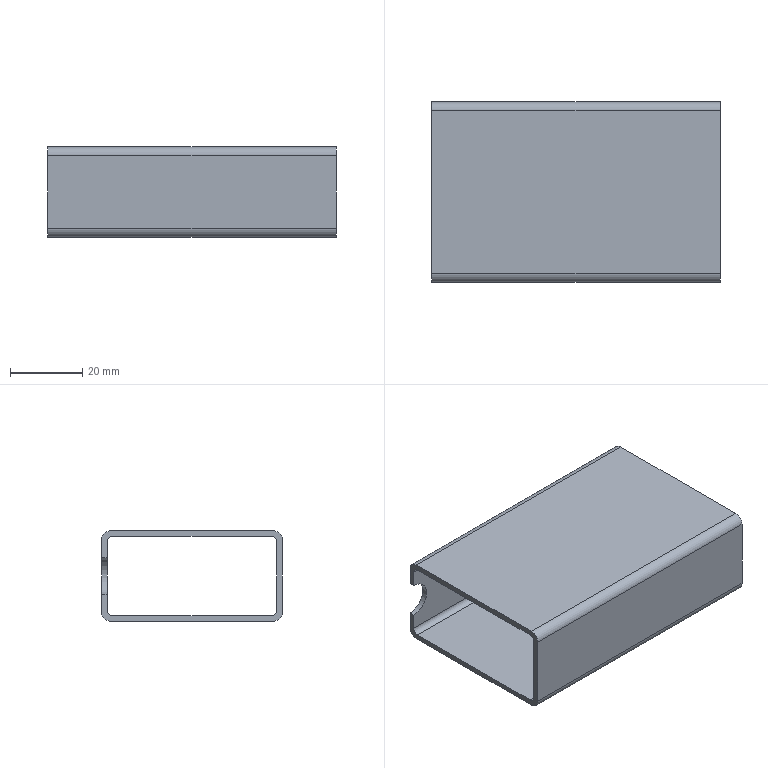Part | STEP file | 6150507 | 1 solid | 19 faces | box 80 x 50 x 25 mm | volume 16946 mm3 | plane 10 | cylinder 9 | commonest cylinder face diameters 3 x4 5 x4 10 x1
STEP:
#1=CARTESIAN_POINT('',(-40.,23.5,-9.5));
#2=VERTEX_POINT('',#1);
#3=CARTESIAN_POINT('',(-40.,23.5,-5.));
#4=VERTEX_POINT('',#3);
#5=CARTESIAN_POINT('',(-40.,23.5,9.5));
#6=DIRECTION('',(0.,0.,1.));
#7=VECTOR('',#6,1000.);
#8=LINE('',#5,#7);
#9=EDGE_CURVE('',#2,#4,#8,.T.);
#10=ORIENTED_EDGE('',*,*,#9,.T.);
#11=CARTESIAN_POINT('',(-40.,25.,-5.));
#12=VERTEX_POINT('',#11);
#13=CARTESIAN_POINT('',(-40.,15.,-5.));
#14=DIRECTION('',(0.,1.,0.));
#15=VECTOR('',#14,1000.);
#16=LINE('',#13,#15);
#17=EDGE_CURVE('',#4,#12,#16,.T.);
#18=ORIENTED_EDGE('',*,*,#17,.T.);
#19=CARTESIAN_POINT('',(-40.,25.,-10.));
#20=VERTEX_POINT('',#19);
#21=CARTESIAN_POINT('',(-40.,25.,12.5));
#22=DIRECTION('',(0.,0.,-1.));
#23=VECTOR('',#22,1000.);
#24=LINE('',#21,#23);
#25=EDGE_CURVE('',#12,#20,#24,.T.);
#26=ORIENTED_EDGE('',*,*,#25,.T.);
#27=CARTESIAN_POINT('',(-40.,22.5,-12.5));
#28=VERTEX_POINT('',#27);
#29=CARTESIAN_POINT('',(-40.,22.5,-10.));
#30=DIRECTION('',(-1.,0.,0.));
#31=DIRECTION('',(0.,1.,0.));
#32=AXIS2_PLACEMENT_3D('',#29,#30,#31);
#33=CIRCLE('',#32,2.5);
#34=EDGE_CURVE('',#20,#28,#33,.T.);
#35=ORIENTED_EDGE('',*,*,#34,.T.);
#36=CARTESIAN_POINT('',(-40.,-22.5,-12.5));
#37=VERTEX_POINT('',#36);
#38=CARTESIAN_POINT('',(-40.,25.,-12.5));
#39=DIRECTION('',(0.,-1.,0.));
#40=VECTOR('',#39,1000.);
#41=LINE('',#38,#40);
#42=EDGE_CURVE('',#28,#37,#41,.T.);
#43=ORIENTED_EDGE('',*,*,#42,.T.);
#44=CARTESIAN_POINT('',(-40.,-25.,-10.));
#45=VERTEX_POINT('',#44);
#46=CARTESIAN_POINT('',(-40.,-22.5,-10.));
#47=DIRECTION('',(-1.,0.,0.));
#48=DIRECTION('',(0.,1.,0.));
#49=AXIS2_PLACEMENT_3D('',#46,#47,#48);
#50=CIRCLE('',#49,2.5);
#51=EDGE_CURVE('',#37,#45,#50,.T.);
#52=ORIENTED_EDGE('',*,*,#51,.T.);
#53=CARTESIAN_POINT('',(-40.,-25.,10.));
#54=VERTEX_POINT('',#53);
#55=CARTESIAN_POINT('',(-40.,-25.,12.5));
#56=DIRECTION('',(0.,0.,-1.));
#57=VECTOR('',#56,1000.);
#58=LINE('',#55,#57);
#59=EDGE_CURVE('',#54,#45,#58,.T.);
#60=ORIENTED_EDGE('',*,*,#59,.F.);
#61=CARTESIAN_POINT('',(-40.,-22.5,12.5));
#62=VERTEX_POINT('',#61);
#63=CARTESIAN_POINT('',(-40.,-22.5,10.));
#64=DIRECTION('',(-1.,0.,0.));
#65=DIRECTION('',(0.,1.,0.));
#66=AXIS2_PLACEMENT_3D('',#63,#64,#65);
#67=CIRCLE('',#66,2.5);
#68=EDGE_CURVE('',#54,#62,#67,.T.);
#69=ORIENTED_EDGE('',*,*,#68,.T.);
#70=CARTESIAN_POINT('',(-40.,22.5,12.5));
#71=VERTEX_POINT('',#70);
#72=CARTESIAN_POINT('',(-40.,25.,12.5));
#73=DIRECTION('',(0.,-1.,0.));
#74=VECTOR('',#73,1000.);
#75=LINE('',#72,#74);
#76=EDGE_CURVE('',#71,#62,#75,.T.);
#77=ORIENTED_EDGE('',*,*,#76,.F.);
#78=CARTESIAN_POINT('',(-40.,25.,10.));
#79=VERTEX_POINT('',#78);
#80=CARTESIAN_POINT('',(-40.,22.5,10.));
#81=DIRECTION('',(-1.,0.,0.));
#82=DIRECTION('',(0.,1.,0.));
#83=AXIS2_PLACEMENT_3D('',#80,#81,#82);
#84=CIRCLE('',#83,2.5);
#85=EDGE_CURVE('',#71,#79,#84,.T.);
#86=ORIENTED_EDGE('',*,*,#85,.T.);
#87=CARTESIAN_POINT('',(-40.,25.,5.));
#88=VERTEX_POINT('',#87);
#89=CARTESIAN_POINT('',(-40.,25.,12.5));
#90=DIRECTION('',(0.,0.,-1.));
#91=VECTOR('',#90,1000.);
#92=LINE('',#89,#91);
#93=EDGE_CURVE('',#79,#88,#92,.T.);
#94=ORIENTED_EDGE('',*,*,#93,.T.);
#95=CARTESIAN_POINT('',(-40.,23.5,5.));
#96=VERTEX_POINT('',#95);
#97=CARTESIAN_POINT('',(-40.,15.,5.));
#98=DIRECTION('',(0.,-1.,0.));
#99=VECTOR('',#98,1000.);
#100=LINE('',#97,#99);
#101=EDGE_CURVE('',#88,#96,#100,.T.);
#102=ORIENTED_EDGE('',*,*,#101,.T.);
#103=CARTESIAN_POINT('',(-40.,23.5,9.5));
#104=VERTEX_POINT('',#103);
#105=CARTESIAN_POINT('',(-40.,23.5,9.5));
#106=DIRECTION('',(0.,0.,1.));
#107=VECTOR('',#106,1000.);
#108=LINE('',#105,#107);
#109=EDGE_CURVE('',#96,#104,#108,.T.);
#110=ORIENTED_EDGE('',*,*,#109,.T.);
#111=CARTESIAN_POINT('',(-40.,22.,11.));
#112=VERTEX_POINT('',#111);
#113=CARTESIAN_POINT('',(-40.,22.,9.5));
#114=DIRECTION('',(1.,0.,0.));
#115=DIRECTION('',(0.,1.,0.));
#116=AXIS2_PLACEMENT_3D('',#113,#114,#115);
#117=CIRCLE('',#116,1.5);
#118=EDGE_CURVE('',#104,#112,#117,.T.);
#119=ORIENTED_EDGE('',*,*,#118,.T.);
#120=CARTESIAN_POINT('',(-40.,-22.,11.));
#121=VERTEX_POINT('',#120);
#122=CARTESIAN_POINT('',(-40.,22.,11.));
#123=DIRECTION('',(0.,-1.,0.));
#124=VECTOR('',#123,1000.);
#125=LINE('',#122,#124);
#126=EDGE_CURVE('',#112,#121,#125,.T.);
#127=ORIENTED_EDGE('',*,*,#126,.T.);
#128=CARTESIAN_POINT('',(-40.,-23.5,9.5));
#129=VERTEX_POINT('',#128);
#130=CARTESIAN_POINT('',(-40.,-22.,9.5));
#131=DIRECTION('',(1.,0.,0.));
#132=DIRECTION('',(0.,1.,0.));
#133=AXIS2_PLACEMENT_3D('',#130,#131,#132);
#134=CIRCLE('',#133,1.5);
#135=EDGE_CURVE('',#121,#129,#134,.T.);
#136=ORIENTED_EDGE('',*,*,#135,.T.);
#137=CARTESIAN_POINT('',(-40.,-23.5,-9.5));
#138=VERTEX_POINT('',#137);
#139=CARTESIAN_POINT('',(-40.,-23.5,9.5));
#140=DIRECTION('',(0.,0.,-1.));
#141=VECTOR('',#140,1000.);
#142=LINE('',#139,#141);
#143=EDGE_CURVE('',#129,#138,#142,.T.);
#144=ORIENTED_EDGE('',*,*,#143,.T.);
#145=CARTESIAN_POINT('',(-40.,-22.,-11.));
#146=VERTEX_POINT('',#145);
#147=CARTESIAN_POINT('',(-40.,-22.,-9.5));
#148=DIRECTION('',(1.,0.,0.));
#149=DIRECTION('',(0.,1.,0.));
#150=AXIS2_PLACEMENT_3D('',#147,#148,#149);
#151=CIRCLE('',#150,1.5);
#152=EDGE_CURVE('',#138,#146,#151,.T.);
#153=ORIENTED_EDGE('',*,*,#152,.T.);
#154=CARTESIAN_POINT('',(-40.,22.,-11.));
#155=VERTEX_POINT('',#154);
#156=CARTESIAN_POINT('',(-40.,22.,-11.));
#157=DIRECTION('',(0.,1.,0.));
#158=VECTOR('',#157,1000.);
#159=LINE('',#156,#158);
#160=EDGE_CURVE('',#146,#155,#159,.T.);
#161=ORIENTED_EDGE('',*,*,#160,.T.);
#162=CARTESIAN_POINT('',(-40.,22.,-9.5));
#163=DIRECTION('',(1.,0.,0.));
#164=DIRECTION('',(0.,-1.,0.));
#165=AXIS2_PLACEMENT_3D('',#162,#163,#164);
#166=CIRCLE('',#165,1.5);
#167=EDGE_CURVE('',#155,#2,#166,.T.);
#168=ORIENTED_EDGE('',*,*,#167,.T.);
#169=EDGE_LOOP('',(#10,#18,#26,#35,#43,#52,#60,#69,#77,#86,#94,#102,#110,#119,#127,#136,#144,#153,#161,#168));
#170=FACE_OUTER_BOUND('',#169,.T.);
#171=CARTESIAN_POINT('',(-40.,25.,12.5));
#172=DIRECTION('',(1.,0.,0.));
#173=DIRECTION('',(0.,1.,0.));
#174=AXIS2_PLACEMENT_3D('',#171,#172,#173);
#175=PLANE('',#174);
#176=ADVANCED_FACE('',(#170),#175,.F.);
#177=CARTESIAN_POINT('',(40.,-25.,10.));
#178=VERTEX_POINT('',#177);
#179=CARTESIAN_POINT('',(40.,-25.,-10.));
#180=VERTEX_POINT('',#179);
#181=CARTESIAN_POINT('',(40.,-25.,12.5));
#182=DIRECTION('',(0.,0.,-1.));
#183=VECTOR('',#182,1000.);
#184=LINE('',#181,#183);
#185=EDGE_CURVE('',#178,#180,#184,.T.);
#186=ORIENTED_EDGE('',*,*,#185,.F.);
#187=CARTESIAN_POINT('',(-40.,-25.,10.));
#188=DIRECTION('',(-1.,0.,0.));
#189=VECTOR('',#188,1000.);
#190=LINE('',#187,#189);
#191=EDGE_CURVE('',#178,#54,#190,.T.);
#192=ORIENTED_EDGE('',*,*,#191,.T.);
#193=ORIENTED_EDGE('',*,*,#59,.T.);
#194=CARTESIAN_POINT('',(-40.,-25.,-10.));
#195=DIRECTION('',(1.,0.,0.));
#196=VECTOR('',#195,1000.);
#197=LINE('',#194,#196);
#198=EDGE_CURVE('',#45,#180,#197,.T.);
#199=ORIENTED_EDGE('',*,*,#198,.T.);
#200=EDGE_LOOP('',(#186,#192,#193,#199));
#201=FACE_OUTER_BOUND('',#200,.T.);
#202=CARTESIAN_POINT('',(-40.,-25.,12.5));
#203=DIRECTION('',(0.,1.,0.));
#204=DIRECTION('',(-1.,0.,0.));
#205=AXIS2_PLACEMENT_3D('',#202,#203,#204);
#206=PLANE('',#205);
#207=ADVANCED_FACE('',(#201),#206,.F.);
#208=CARTESIAN_POINT('',(40.,-23.5,9.5));
#209=VERTEX_POINT('',#208);
#210=CARTESIAN_POINT('',(40.,-23.5,-9.5));
#211=VERTEX_POINT('',#210);
#212=CARTESIAN_POINT('',(40.,-23.5,9.5));
#213=DIRECTION('',(0.,0.,-1.));
#214=VECTOR('',#213,1000.);
#215=LINE('',#212,#214);
#216=EDGE_CURVE('',#209,#211,#215,.T.);
#217=ORIENTED_EDGE('',*,*,#216,.F.);
#218=CARTESIAN_POINT('',(40.,-22.,11.));
#219=VERTEX_POINT('',#218);
#220=CARTESIAN_POINT('',(40.,-22.,9.5));
#221=DIRECTION('',(1.,0.,0.));
#222=DIRECTION('',(0.,1.,0.));
#223=AXIS2_PLACEMENT_3D('',#220,#221,#222);
#224=CIRCLE('',#223,1.5);
#225=EDGE_CURVE('',#219,#209,#224,.T.);
#226=ORIENTED_EDGE('',*,*,#225,.F.);
#227=CARTESIAN_POINT('',(40.,22.,11.));
#228=VERTEX_POINT('',#227);
#229=CARTESIAN_POINT('',(40.,22.,11.));
#230=DIRECTION('',(0.,-1.,0.));
#231=VECTOR('',#230,1000.);
#232=LINE('',#229,#231);
#233=EDGE_CURVE('',#228,#219,#232,.T.);
#234=ORIENTED_EDGE('',*,*,#233,.F.);
#235=CARTESIAN_POINT('',(40.,23.5,9.5));
#236=VERTEX_POINT('',#235);
#237=CARTESIAN_POINT('',(40.,22.,9.5));
#238=DIRECTION('',(1.,0.,0.));
#239=DIRECTION('',(0.,1.,0.));
#240=AXIS2_PLACEMENT_3D('',#237,#238,#239);
#241=CIRCLE('',#240,1.5);
#242=EDGE_CURVE('',#236,#228,#241,.T.);
#243=ORIENTED_EDGE('',*,*,#242,.F.);
#244=CARTESIAN_POINT('',(40.,23.5,-9.5));
#245=VERTEX_POINT('',#244);
#246=CARTESIAN_POINT('',(40.,23.5,9.5));
#247=DIRECTION('',(0.,0.,1.));
#248=VECTOR('',#247,1000.);
#249=LINE('',#246,#248);
#250=EDGE_CURVE('',#245,#236,#249,.T.);
#251=ORIENTED_EDGE('',*,*,#250,.F.);
#252=CARTESIAN_POINT('',(40.,22.,-11.));
#253=VERTEX_POINT('',#252);
#254=CARTESIAN_POINT('',(40.,22.,-9.5));
#255=DIRECTION('',(1.,0.,0.));
#256=DIRECTION('',(0.,-1.,0.));
#257=AXIS2_PLACEMENT_3D('',#254,#255,#256);
#258=CIRCLE('',#257,1.5);
#259=EDGE_CURVE('',#253,#245,#258,.T.);
#260=ORIENTED_EDGE('',*,*,#259,.F.);
#261=CARTESIAN_POINT('',(40.,-22.,-11.));
#262=VERTEX_POINT('',#261);
#263=CARTESIAN_POINT('',(40.,22.,-11.));
#264=DIRECTION('',(0.,1.,0.));
#265=VECTOR('',#264,1000.);
#266=LINE('',#263,#265);
#267=EDGE_CURVE('',#262,#253,#266,.T.);
#268=ORIENTED_EDGE('',*,*,#267,.F.);
#269=CARTESIAN_POINT('',(40.,-22.,-9.5));
#270=DIRECTION('',(1.,0.,0.));
#271=DIRECTION('',(0.,1.,0.));
#272=AXIS2_PLACEMENT_3D('',#269,#270,#271);
#273=CIRCLE('',#272,1.5);
#274=EDGE_CURVE('',#211,#262,#273,.T.);
#275=ORIENTED_EDGE('',*,*,#274,.F.);
#276=EDGE_LOOP('',(#217,#226,#234,#243,#251,#260,#268,#275));
#277=FACE_BOUND('',#276,.T.);
#278=CARTESIAN_POINT('',(40.,-22.5,12.5));
#279=VERTEX_POINT('',#278);
#280=CARTESIAN_POINT('',(40.,22.5,12.5));
#281=VERTEX_POINT('',#280);
#282=CARTESIAN_POINT('',(40.,25.,12.5));
#283=DIRECTION('',(0.,1.,0.));
#284=VECTOR('',#283,1000.);
#285=LINE('',#282,#284);
#286=EDGE_CURVE('',#279,#281,#285,.T.);
#287=ORIENTED_EDGE('',*,*,#286,.F.);
#288=CARTESIAN_POINT('',(40.,-22.5,10.));
#289=DIRECTION('',(1.,0.,0.));
#290=DIRECTION('',(0.,-1.,0.));
#291=AXIS2_PLACEMENT_3D('',#288,#289,#290);
#292=CIRCLE('',#291,2.5);
#293=EDGE_CURVE('',#279,#178,#292,.T.);
#294=ORIENTED_EDGE('',*,*,#293,.T.);
#295=ORIENTED_EDGE('',*,*,#185,.T.);
#296=CARTESIAN_POINT('',(40.,-22.5,-12.5));
#297=VERTEX_POINT('',#296);
#298=CARTESIAN_POINT('',(40.,-22.5,-10.));
#299=DIRECTION('',(1.,0.,0.));
#300=DIRECTION('',(0.,-1.,0.));
#301=AXIS2_PLACEMENT_3D('',#298,#299,#300);
#302=CIRCLE('',#301,2.5);
#303=EDGE_CURVE('',#180,#297,#302,.T.);
#304=ORIENTED_EDGE('',*,*,#303,.T.);
#305=CARTESIAN_POINT('',(40.,22.5,-12.5));
#306=VERTEX_POINT('',#305);
#307=CARTESIAN_POINT('',(40.,25.,-12.5));
#308=DIRECTION('',(0.,1.,0.));
#309=VECTOR('',#308,1000.);
#310=LINE('',#307,#309);
#311=EDGE_CURVE('',#297,#306,#310,.T.);
#312=ORIENTED_EDGE('',*,*,#311,.T.);
#313=CARTESIAN_POINT('',(40.,25.,-10.));
#314=VERTEX_POINT('',#313);
#315=CARTESIAN_POINT('',(40.,22.5,-10.));
#316=DIRECTION('',(1.,0.,0.));
#317=DIRECTION('',(0.,-1.,0.));
#318=AXIS2_PLACEMENT_3D('',#315,#316,#317);
#319=CIRCLE('',#318,2.5);
#320=EDGE_CURVE('',#306,#314,#319,.T.);
#321=ORIENTED_EDGE('',*,*,#320,.T.);
#322=CARTESIAN_POINT('',(40.,25.,10.));
#323=VERTEX_POINT('',#322);
#324=CARTESIAN_POINT('',(40.,25.,12.5));
#325=DIRECTION('',(0.,0.,-1.));
#326=VECTOR('',#325,1000.);
#327=LINE('',#324,#326);
#328=EDGE_CURVE('',#323,#314,#327,.T.);
#329=ORIENTED_EDGE('',*,*,#328,.F.);
#330=CARTESIAN_POINT('',(40.,22.5,10.));
#331=DIRECTION('',(1.,0.,0.));
#332=DIRECTION('',(0.,-1.,0.));
#333=AXIS2_PLACEMENT_3D('',#330,#331,#332);
#334=CIRCLE('',#333,2.5);
#335=EDGE_CURVE('',#323,#281,#334,.T.);
#336=ORIENTED_EDGE('',*,*,#335,.T.);
#337=EDGE_LOOP('',(#287,#294,#295,#304,#312,#321,#329,#336));
#338=FACE_OUTER_BOUND('',#337,.T.);
#339=CARTESIAN_POINT('',(40.,25.,12.5));
#340=DIRECTION('',(-1.,0.,0.));
#341=DIRECTION('',(0.,-1.,0.));
#342=AXIS2_PLACEMENT_3D('',#339,#340,#341);
#343=PLANE('',#342);
#344=ADVANCED_FACE('',(#277,#338),#343,.F.);
#345=ORIENTED_EDGE('',*,*,#25,.F.);
#346=CARTESIAN_POINT('',(-40.,25.,0.));
#347=DIRECTION('',(0.,1.,0.));
#348=DIRECTION('',(0.,0.,1.));
#349=AXIS2_PLACEMENT_3D('',#346,#347,#348);
#350=CIRCLE('',#349,5.);
#351=EDGE_CURVE('',#88,#12,#350,.T.);
#352=ORIENTED_EDGE('',*,*,#351,.F.);
#353=ORIENTED_EDGE('',*,*,#93,.F.);
#354=CARTESIAN_POINT('',(40.,25.,10.));
#355=DIRECTION('',(1.,0.,0.));
#356=VECTOR('',#355,1000.);
#357=LINE('',#354,#356);
#358=EDGE_CURVE('',#79,#323,#357,.T.);
#359=ORIENTED_EDGE('',*,*,#358,.T.);
#360=ORIENTED_EDGE('',*,*,#328,.T.);
#361=CARTESIAN_POINT('',(-40.,25.,-10.));
#362=DIRECTION('',(-1.,0.,0.));
#363=VECTOR('',#362,1000.);
#364=LINE('',#361,#363);
#365=EDGE_CURVE('',#314,#20,#364,.T.);
#366=ORIENTED_EDGE('',*,*,#365,.T.);
#367=EDGE_LOOP('',(#345,#352,#353,#359,#360,#366));
#368=FACE_OUTER_BOUND('',#367,.T.);
#369=CARTESIAN_POINT('',(-40.,25.,12.5));
#370=DIRECTION('',(0.,-1.,0.));
#371=DIRECTION('',(0.,0.,-1.));
#372=AXIS2_PLACEMENT_3D('',#369,#370,#371);
#373=PLANE('',#372);
#374=ADVANCED_FACE('',(#368),#373,.F.);
#375=ORIENTED_EDGE('',*,*,#76,.T.);
#376=CARTESIAN_POINT('',(40.,-22.5,12.5));
#377=DIRECTION('',(1.,0.,0.));
#378=VECTOR('',#377,1000.);
#379=LINE('',#376,#378);
#380=EDGE_CURVE('',#62,#279,#379,.T.);
#381=ORIENTED_EDGE('',*,*,#380,.T.);
#382=ORIENTED_EDGE('',*,*,#286,.T.);
#383=CARTESIAN_POINT('',(-40.,22.5,12.5));
#384=DIRECTION('',(-1.,0.,0.));
#385=VECTOR('',#384,1000.);
#386=LINE('',#383,#385);
#387=EDGE_CURVE('',#281,#71,#386,.T.);
#388=ORIENTED_EDGE('',*,*,#387,.T.);
#389=EDGE_LOOP('',(#375,#381,#382,#388));
#390=FACE_OUTER_BOUND('',#389,.T.);
#391=CARTESIAN_POINT('',(-40.,-25.,12.5));
#392=DIRECTION('',(0.,0.,1.));
#393=DIRECTION('',(1.,0.,0.));
#394=AXIS2_PLACEMENT_3D('',#391,#392,#393);
#395=PLANE('',#394);
#396=ADVANCED_FACE('',(#390),#395,.T.);
#397=ORIENTED_EDGE('',*,*,#311,.F.);
#398=CARTESIAN_POINT('',(-40.,-22.5,-12.5));
#399=DIRECTION('',(-1.,0.,0.));
#400=VECTOR('',#399,1000.);
#401=LINE('',#398,#400);
#402=EDGE_CURVE('',#297,#37,#401,.T.);
#403=ORIENTED_EDGE('',*,*,#402,.T.);
#404=ORIENTED_EDGE('',*,*,#42,.F.);
#405=CARTESIAN_POINT('',(-40.,22.5,-12.5));
#406=DIRECTION('',(1.,0.,0.));
#407=VECTOR('',#406,1000.);
#408=LINE('',#405,#407);
#409=EDGE_CURVE('',#28,#306,#408,.T.);
#410=ORIENTED_EDGE('',*,*,#409,.T.);
#411=EDGE_LOOP('',(#397,#403,#404,#410));
#412=FACE_OUTER_BOUND('',#411,.T.);
#413=CARTESIAN_POINT('',(-40.,-25.,-12.5));
#414=DIRECTION('',(0.,0.,1.));
#415=DIRECTION('',(1.,0.,0.));
#416=AXIS2_PLACEMENT_3D('',#413,#414,#415);
#417=PLANE('',#416);
#418=ADVANCED_FACE('',(#412),#417,.F.);
#419=ORIENTED_EDGE('',*,*,#68,.F.);
#420=ORIENTED_EDGE('',*,*,#191,.F.);
#421=ORIENTED_EDGE('',*,*,#293,.F.);
#422=ORIENTED_EDGE('',*,*,#380,.F.);
#423=EDGE_LOOP('',(#419,#420,#421,#422));
#424=FACE_OUTER_BOUND('',#423,.T.);
#425=CARTESIAN_POINT('',(-40.,-22.5,10.));
#426=DIRECTION('',(-1.,0.,0.));
#427=DIRECTION('',(0.,-1.,0.));
#428=AXIS2_PLACEMENT_3D('',#425,#426,#427);
#429=CYLINDRICAL_SURFACE('',#428,2.5);
#430=ADVANCED_FACE('',(#424),#429,.T.);
#431=ORIENTED_EDGE('',*,*,#51,.F.);
#432=ORIENTED_EDGE('',*,*,#402,.F.);
#433=ORIENTED_EDGE('',*,*,#303,.F.);
#434=ORIENTED_EDGE('',*,*,#198,.F.);
#435=EDGE_LOOP('',(#431,#432,#433,#434));
#436=FACE_OUTER_BOUND('',#435,.T.);
#437=CARTESIAN_POINT('',(-40.,-22.5,-10.));
#438=DIRECTION('',(1.,0.,0.));
#439=DIRECTION('',(0.,1.,0.));
#440=AXIS2_PLACEMENT_3D('',#437,#438,#439);
#441=CYLINDRICAL_SURFACE('',#440,2.5);
#442=ADVANCED_FACE('',(#436),#441,.T.);
#443=ORIENTED_EDGE('',*,*,#320,.F.);
#444=ORIENTED_EDGE('',*,*,#409,.F.);
#445=ORIENTED_EDGE('',*,*,#34,.F.);
#446=ORIENTED_EDGE('',*,*,#365,.F.);
#447=EDGE_LOOP('',(#443,#444,#445,#446));
#448=FACE_OUTER_BOUND('',#447,.T.);
#449=CARTESIAN_POINT('',(-40.,22.5,-10.));
#450=DIRECTION('',(-1.,0.,0.));
#451=DIRECTION('',(0.,0.,1.));
#452=AXIS2_PLACEMENT_3D('',#449,#450,#451);
#453=CYLINDRICAL_SURFACE('',#452,2.5);
#454=ADVANCED_FACE('',(#448),#453,.T.);
#455=ORIENTED_EDGE('',*,*,#335,.F.);
#456=ORIENTED_EDGE('',*,*,#358,.F.);
#457=ORIENTED_EDGE('',*,*,#85,.F.);
#458=ORIENTED_EDGE('',*,*,#387,.F.);
#459=EDGE_LOOP('',(#455,#456,#457,#458));
#460=FACE_OUTER_BOUND('',#459,.T.);
#461=CARTESIAN_POINT('',(-40.,22.5,10.));
#462=DIRECTION('',(1.,0.,0.));
#463=DIRECTION('',(0.,0.,-1.));
#464=AXIS2_PLACEMENT_3D('',#461,#462,#463);
#465=CYLINDRICAL_SURFACE('',#464,2.5);
#466=ADVANCED_FACE('',(#460),#465,.T.);
#467=ORIENTED_EDGE('',*,*,#225,.T.);
#468=CARTESIAN_POINT('',(-40.,-23.5,9.5));
#469=DIRECTION('',(1.,0.,0.));
#470=VECTOR('',#469,1000.);
#471=LINE('',#468,#470);
#472=EDGE_CURVE('',#129,#209,#471,.T.);
#473=ORIENTED_EDGE('',*,*,#472,.F.);
#474=ORIENTED_EDGE('',*,*,#135,.F.);
#475=CARTESIAN_POINT('',(-40.,-22.,11.));
#476=DIRECTION('',(1.,0.,0.));
#477=VECTOR('',#476,1000.);
#478=LINE('',#475,#477);
#479=EDGE_CURVE('',#121,#219,#478,.T.);
#480=ORIENTED_EDGE('',*,*,#479,.T.);
#481=EDGE_LOOP('',(#467,#473,#474,#480));
#482=FACE_OUTER_BOUND('',#481,.T.);
#483=CARTESIAN_POINT('',(-40.,-22.,9.5));
#484=DIRECTION('',(1.,0.,0.));
#485=DIRECTION('',(0.,1.,0.));
#486=AXIS2_PLACEMENT_3D('',#483,#484,#485);
#487=CYLINDRICAL_SURFACE('',#486,1.5);
#488=ADVANCED_FACE('',(#482),#487,.F.);
#489=ORIENTED_EDGE('',*,*,#233,.T.);
#490=ORIENTED_EDGE('',*,*,#479,.F.);
#491=ORIENTED_EDGE('',*,*,#126,.F.);
#492=CARTESIAN_POINT('',(-40.,22.,11.));
#493=DIRECTION('',(1.,0.,0.));
#494=VECTOR('',#493,1000.);
#495=LINE('',#492,#494);
#496=EDGE_CURVE('',#112,#228,#495,.T.);
#497=ORIENTED_EDGE('',*,*,#496,.T.);
#498=EDGE_LOOP('',(#489,#490,#491,#497));
#499=FACE_OUTER_BOUND('',#498,.T.);
#500=CARTESIAN_POINT('',(-40.,22.,11.));
#501=DIRECTION('',(0.,0.,1.));
#502=DIRECTION('',(0.,-1.,0.));
#503=AXIS2_PLACEMENT_3D('',#500,#501,#502);
#504=PLANE('',#503);
#505=ADVANCED_FACE('',(#499),#504,.F.);
#506=ORIENTED_EDGE('',*,*,#242,.T.);
#507=ORIENTED_EDGE('',*,*,#496,.F.);
#508=ORIENTED_EDGE('',*,*,#118,.F.);
#509=CARTESIAN_POINT('',(-40.,23.5,9.5));
#510=DIRECTION('',(1.,0.,0.));
#511=VECTOR('',#510,1000.);
#512=LINE('',#509,#511);
#513=EDGE_CURVE('',#104,#236,#512,.T.);
#514=ORIENTED_EDGE('',*,*,#513,.T.);
#515=EDGE_LOOP('',(#506,#507,#508,#514));
#516=FACE_OUTER_BOUND('',#515,.T.);
#517=CARTESIAN_POINT('',(-40.,22.,9.5));
#518=DIRECTION('',(1.,0.,0.));
#519=DIRECTION('',(0.,1.,0.));
#520=AXIS2_PLACEMENT_3D('',#517,#518,#519);
#521=CYLINDRICAL_SURFACE('',#520,1.5);
#522=ADVANCED_FACE('',(#516),#521,.F.);
#523=ORIENTED_EDGE('',*,*,#109,.F.);
#524=CARTESIAN_POINT('',(-40.,23.5,0.));
#525=DIRECTION('',(0.,1.,0.));
#526=DIRECTION('',(-1.,0.,0.));
#527=AXIS2_PLACEMENT_3D('',#524,#525,#526);
#528=CIRCLE('',#527,5.);
#529=EDGE_CURVE('',#96,#4,#528,.T.);
#530=ORIENTED_EDGE('',*,*,#529,.T.);
#531=ORIENTED_EDGE('',*,*,#9,.F.);
#532=CARTESIAN_POINT('',(-40.,23.5,-9.5));
#533=DIRECTION('',(1.,0.,0.));
#534=VECTOR('',#533,1000.);
#535=LINE('',#532,#534);
#536=EDGE_CURVE('',#2,#245,#535,.T.);
#537=ORIENTED_EDGE('',*,*,#536,.T.);
#538=ORIENTED_EDGE('',*,*,#250,.T.);
#539=ORIENTED_EDGE('',*,*,#513,.F.);
#540=EDGE_LOOP('',(#523,#530,#531,#537,#538,#539));
#541=FACE_OUTER_BOUND('',#540,.T.);
#542=CARTESIAN_POINT('',(-40.,23.5,9.5));
#543=DIRECTION('',(0.,1.,0.));
#544=DIRECTION('',(-1.,0.,0.));
#545=AXIS2_PLACEMENT_3D('',#542,#543,#544);
#546=PLANE('',#545);
#547=ADVANCED_FACE('',(#541),#546,.F.);
#548=ORIENTED_EDGE('',*,*,#259,.T.);
#549=ORIENTED_EDGE('',*,*,#536,.F.);
#550=ORIENTED_EDGE('',*,*,#167,.F.);
#551=CARTESIAN_POINT('',(-40.,22.,-11.));
#552=DIRECTION('',(1.,0.,0.));
#553=VECTOR('',#552,1000.);
#554=LINE('',#551,#553);
#555=EDGE_CURVE('',#155,#253,#554,.T.);
#556=ORIENTED_EDGE('',*,*,#555,.T.);
#557=EDGE_LOOP('',(#548,#549,#550,#556));
#558=FACE_OUTER_BOUND('',#557,.T.);
#559=CARTESIAN_POINT('',(-40.,22.,-9.5));
#560=DIRECTION('',(1.,0.,0.));
#561=DIRECTION('',(0.,1.,0.));
#562=AXIS2_PLACEMENT_3D('',#559,#560,#561);
#563=CYLINDRICAL_SURFACE('',#562,1.5);
#564=ADVANCED_FACE('',(#558),#563,.F.);
#565=ORIENTED_EDGE('',*,*,#267,.T.);
#566=ORIENTED_EDGE('',*,*,#555,.F.);
#567=ORIENTED_EDGE('',*,*,#160,.F.);
#568=CARTESIAN_POINT('',(-40.,-22.,-11.));
#569=DIRECTION('',(1.,0.,0.));
#570=VECTOR('',#569,1000.);
#571=LINE('',#568,#570);
#572=EDGE_CURVE('',#146,#262,#571,.T.);
#573=ORIENTED_EDGE('',*,*,#572,.T.);
#574=EDGE_LOOP('',(#565,#566,#567,#573));
#575=FACE_OUTER_BOUND('',#574,.T.);
#576=CARTESIAN_POINT('',(-40.,22.,-11.));
#577=DIRECTION('',(0.,0.,-1.));
#578=DIRECTION('',(0.,1.,0.));
#579=AXIS2_PLACEMENT_3D('',#576,#577,#578);
#580=PLANE('',#579);
#581=ADVANCED_FACE('',(#575),#580,.F.);
#582=ORIENTED_EDGE('',*,*,#274,.T.);
#583=ORIENTED_EDGE('',*,*,#572,.F.);
#584=ORIENTED_EDGE('',*,*,#152,.F.);
#585=CARTESIAN_POINT('',(-40.,-23.5,-9.5));
#586=DIRECTION('',(1.,0.,0.));
#587=VECTOR('',#586,1000.);
#588=LINE('',#585,#587);
#589=EDGE_CURVE('',#138,#211,#588,.T.);
#590=ORIENTED_EDGE('',*,*,#589,.T.);
#591=EDGE_LOOP('',(#582,#583,#584,#590));
#592=FACE_OUTER_BOUND('',#591,.T.);
#593=CARTESIAN_POINT('',(-40.,-22.,-9.5));
#594=DIRECTION('',(1.,0.,0.));
#595=DIRECTION('',(0.,1.,0.));
#596=AXIS2_PLACEMENT_3D('',#593,#594,#595);
#597=CYLINDRICAL_SURFACE('',#596,1.5);
#598=ADVANCED_FACE('',(#592),#597,.F.);
#599=ORIENTED_EDGE('',*,*,#216,.T.);
#600=ORIENTED_EDGE('',*,*,#589,.F.);
#601=ORIENTED_EDGE('',*,*,#143,.F.);
#602=ORIENTED_EDGE('',*,*,#472,.T.);
#603=EDGE_LOOP('',(#599,#600,#601,#602));
#604=FACE_OUTER_BOUND('',#603,.T.);
#605=CARTESIAN_POINT('',(-40.,-23.5,9.5));
#606=DIRECTION('',(0.,-1.,0.));
#607=DIRECTION('',(1.,0.,0.));
#608=AXIS2_PLACEMENT_3D('',#605,#606,#607);
#609=PLANE('',#608);
#610=ADVANCED_FACE('',(#604),#609,.F.);
#611=ORIENTED_EDGE('',*,*,#529,.F.);
#612=ORIENTED_EDGE('',*,*,#101,.F.);
#613=ORIENTED_EDGE('',*,*,#351,.T.);
#614=ORIENTED_EDGE('',*,*,#17,.F.);
#615=EDGE_LOOP('',(#611,#612,#613,#614));
#616=FACE_OUTER_BOUND('',#615,.T.);
#617=CARTESIAN_POINT('',(-40.,15.,0.));
#618=DIRECTION('',(0.,1.,0.));
#619=DIRECTION('',(0.,0.,1.));
#620=AXIS2_PLACEMENT_3D('',#617,#618,#619);
#621=CYLINDRICAL_SURFACE('',#620,5.);
#622=ADVANCED_FACE('',(#616),#621,.F.);
#623=CLOSED_SHELL('',(#176,#207,#344,#374,#396,#418,#430,#442,#454,#466,#488,#505,#522,#547,#564,#581,#598,#610,#622));
#624=MANIFOLD_SOLID_BREP('',#623);
#625=CARTESIAN_POINT('',(0.,0.,0.));
#626=DIRECTION('',(0.,0.,1.));
#627=DIRECTION('',(1.,0.,0.));
#628=AXIS2_PLACEMENT_3D('',#625,#626,#627);
#629=(LENGTH_UNIT()NAMED_UNIT(*)SI_UNIT(.MILLI.,.METRE.));
#630=UNCERTAINTY_MEASURE_WITH_UNIT(LENGTH_MEASURE(0.00001),#629,'','');
#631=(NAMED_UNIT(*)PLANE_ANGLE_UNIT()SI_UNIT($,.RADIAN.));
#632=(NAMED_UNIT(*)SI_UNIT($,.STERADIAN.)SOLID_ANGLE_UNIT());
#633=(GEOMETRIC_REPRESENTATION_CONTEXT(3)GLOBAL_UNCERTAINTY_ASSIGNED_CONTEXT((#630))GLOBAL_UNIT_ASSIGNED_CONTEXT((#629,#631,#632))REPRESENTATION_CONTEXT('',''));
#634=ADVANCED_BREP_SHAPE_REPRESENTATION('',(#624,#628),#633);